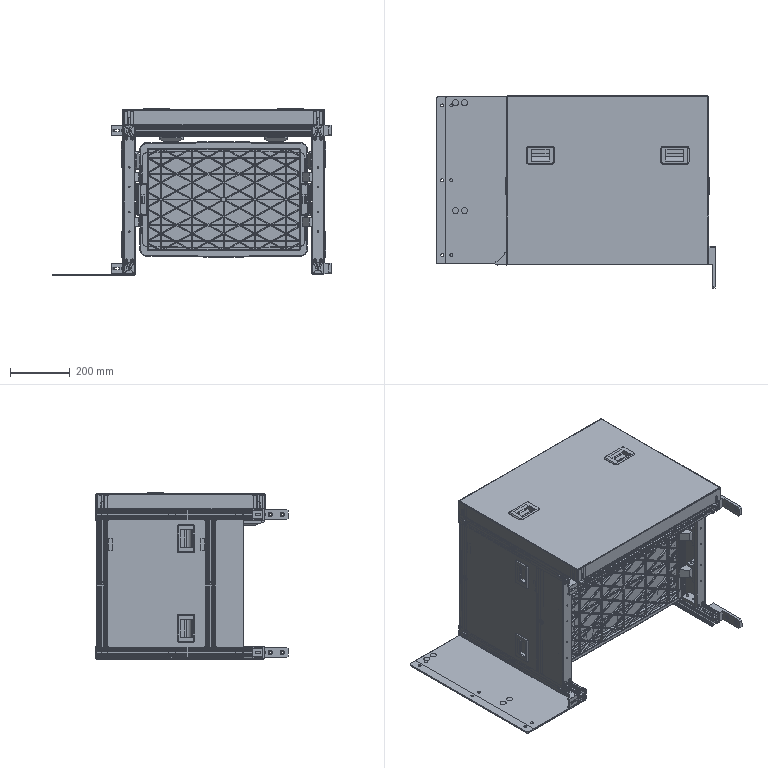Part | SolidWorks | 143 solids | 19190 faces | volume 17249504 mm3 | plane 12015 | cylinder 3828 | spline 1692 | cone 1335 | torus 294 | sphere 26 | commonest cylinder face diameters 4 x666 2 x546 1 x444 0.3 x288 79 x288 9 x204